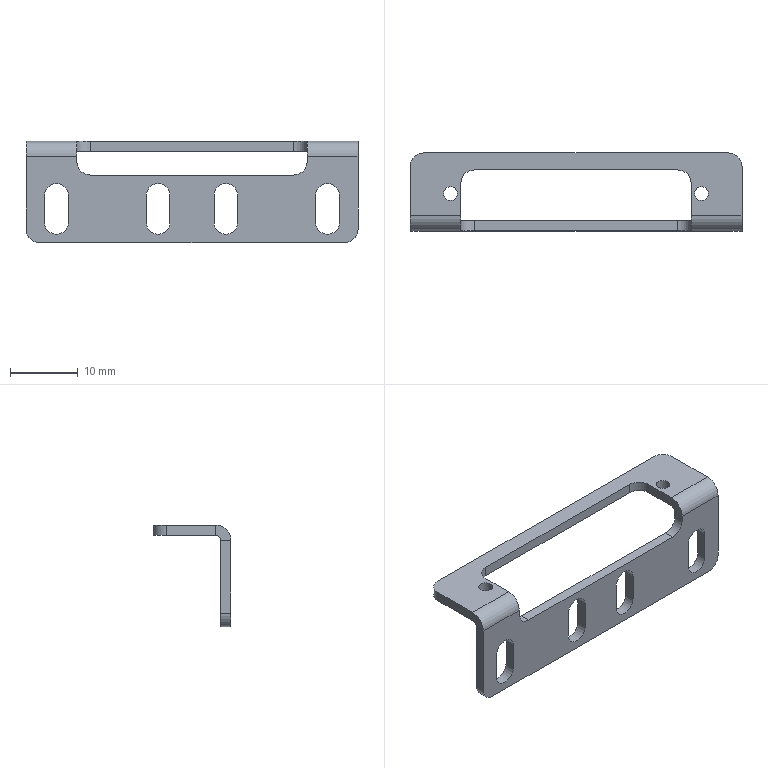Part | STEP file | 07-08LED安装Plate(Default) | 1 solid | 52 faces | box 49 x 11.5 x 15 mm | volume 1034 mm3 | cylinder 28 | plane 24 | commonest cylinder face diameters 3.5 x12 4 x8 2.05 x4 1.473 x2 4.473 x2